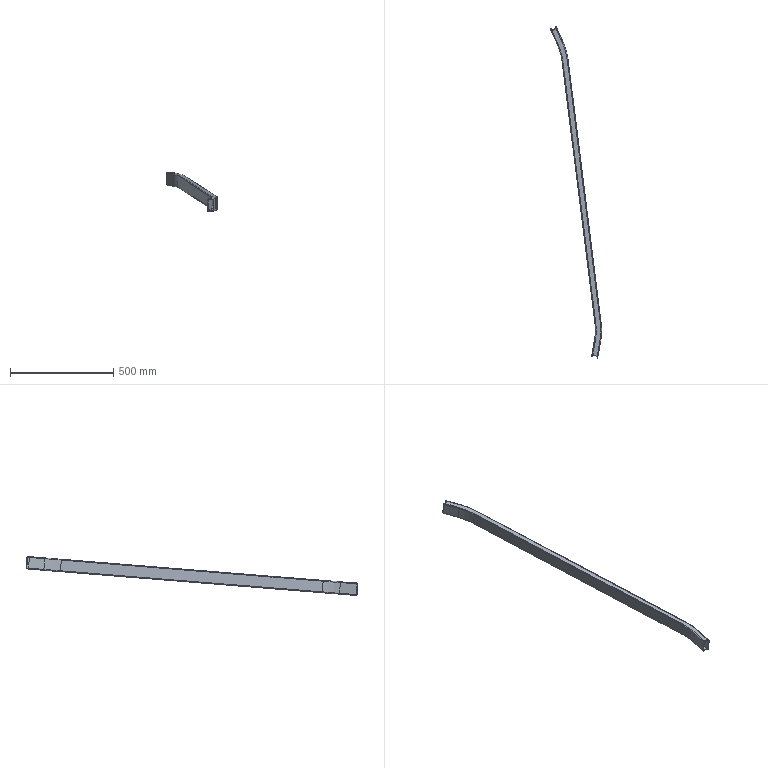Part | SolidWorks | features BaseBody 1 | 1 solid | 99 faces | box 248.187 x 1610 x 188.463 mm | volume 531554 mm3 | cylinder 59 | plane 24 | torus 16 | commonest cylinder face diameters 4 x24 8 x24 33.7 x3 570 x2 574 x2 626 x2